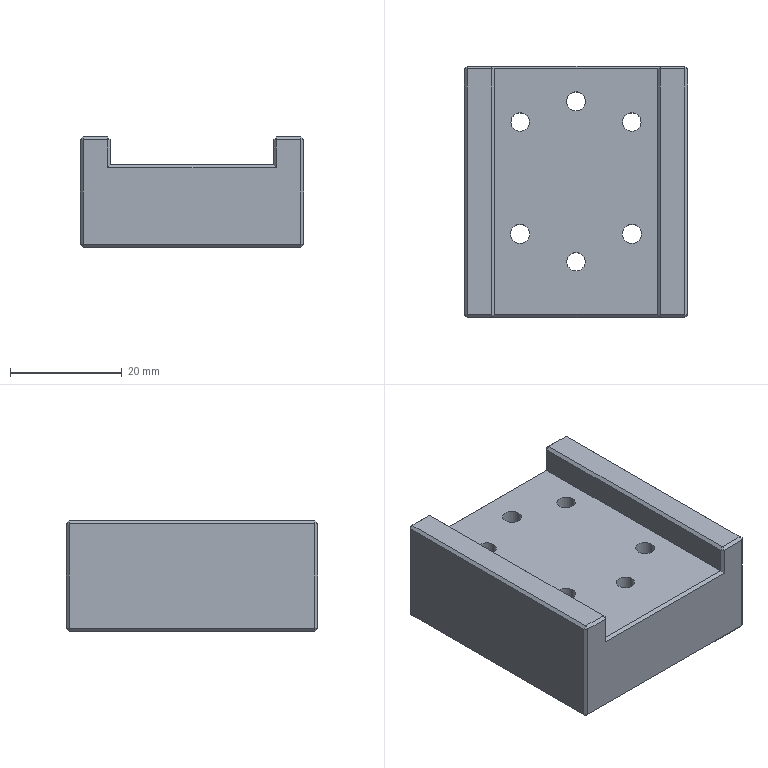Part | SolidWorks | features MirrorStock 1 | 1 solid | 65 faces | box 40 x 45 x 19.7 mm | volume 27758 mm3 | plane 47 | cylinder 18 | commonest cylinder face diameters 3.3 x6 3.4 x6 6.5 x6